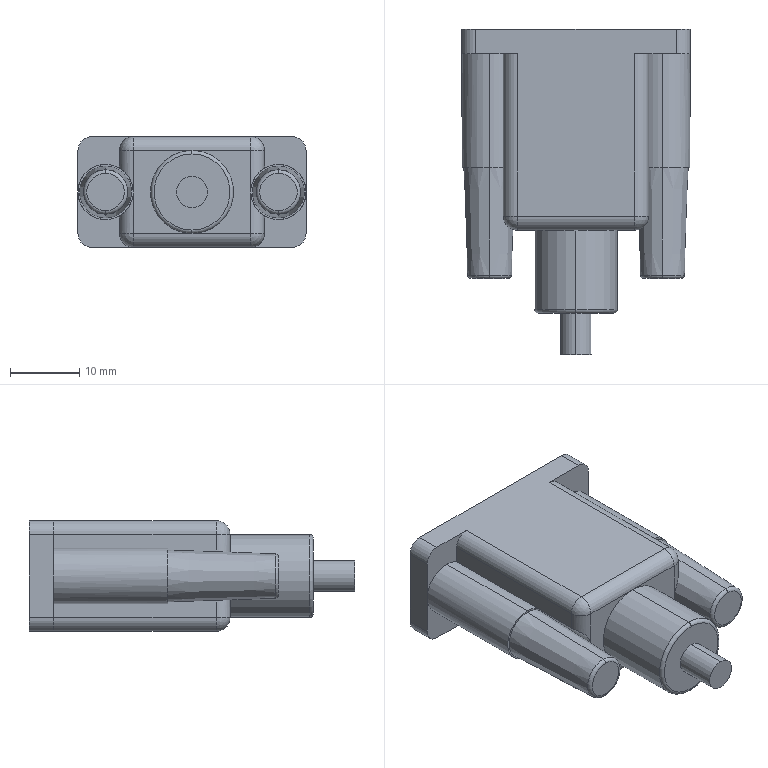Part | SolidWorks | features ICE 5, Fillet 2, Extrusion 1 | 1 solid | 61 faces | box 33 x 47 x 16 mm | volume 14089 mm3 | cylinder 26 | plane 21 | torus 6 | cone 4 | sphere 4 | commonest cylinder face diameters 4 x14 8 x8 4.5 x2 12 x2